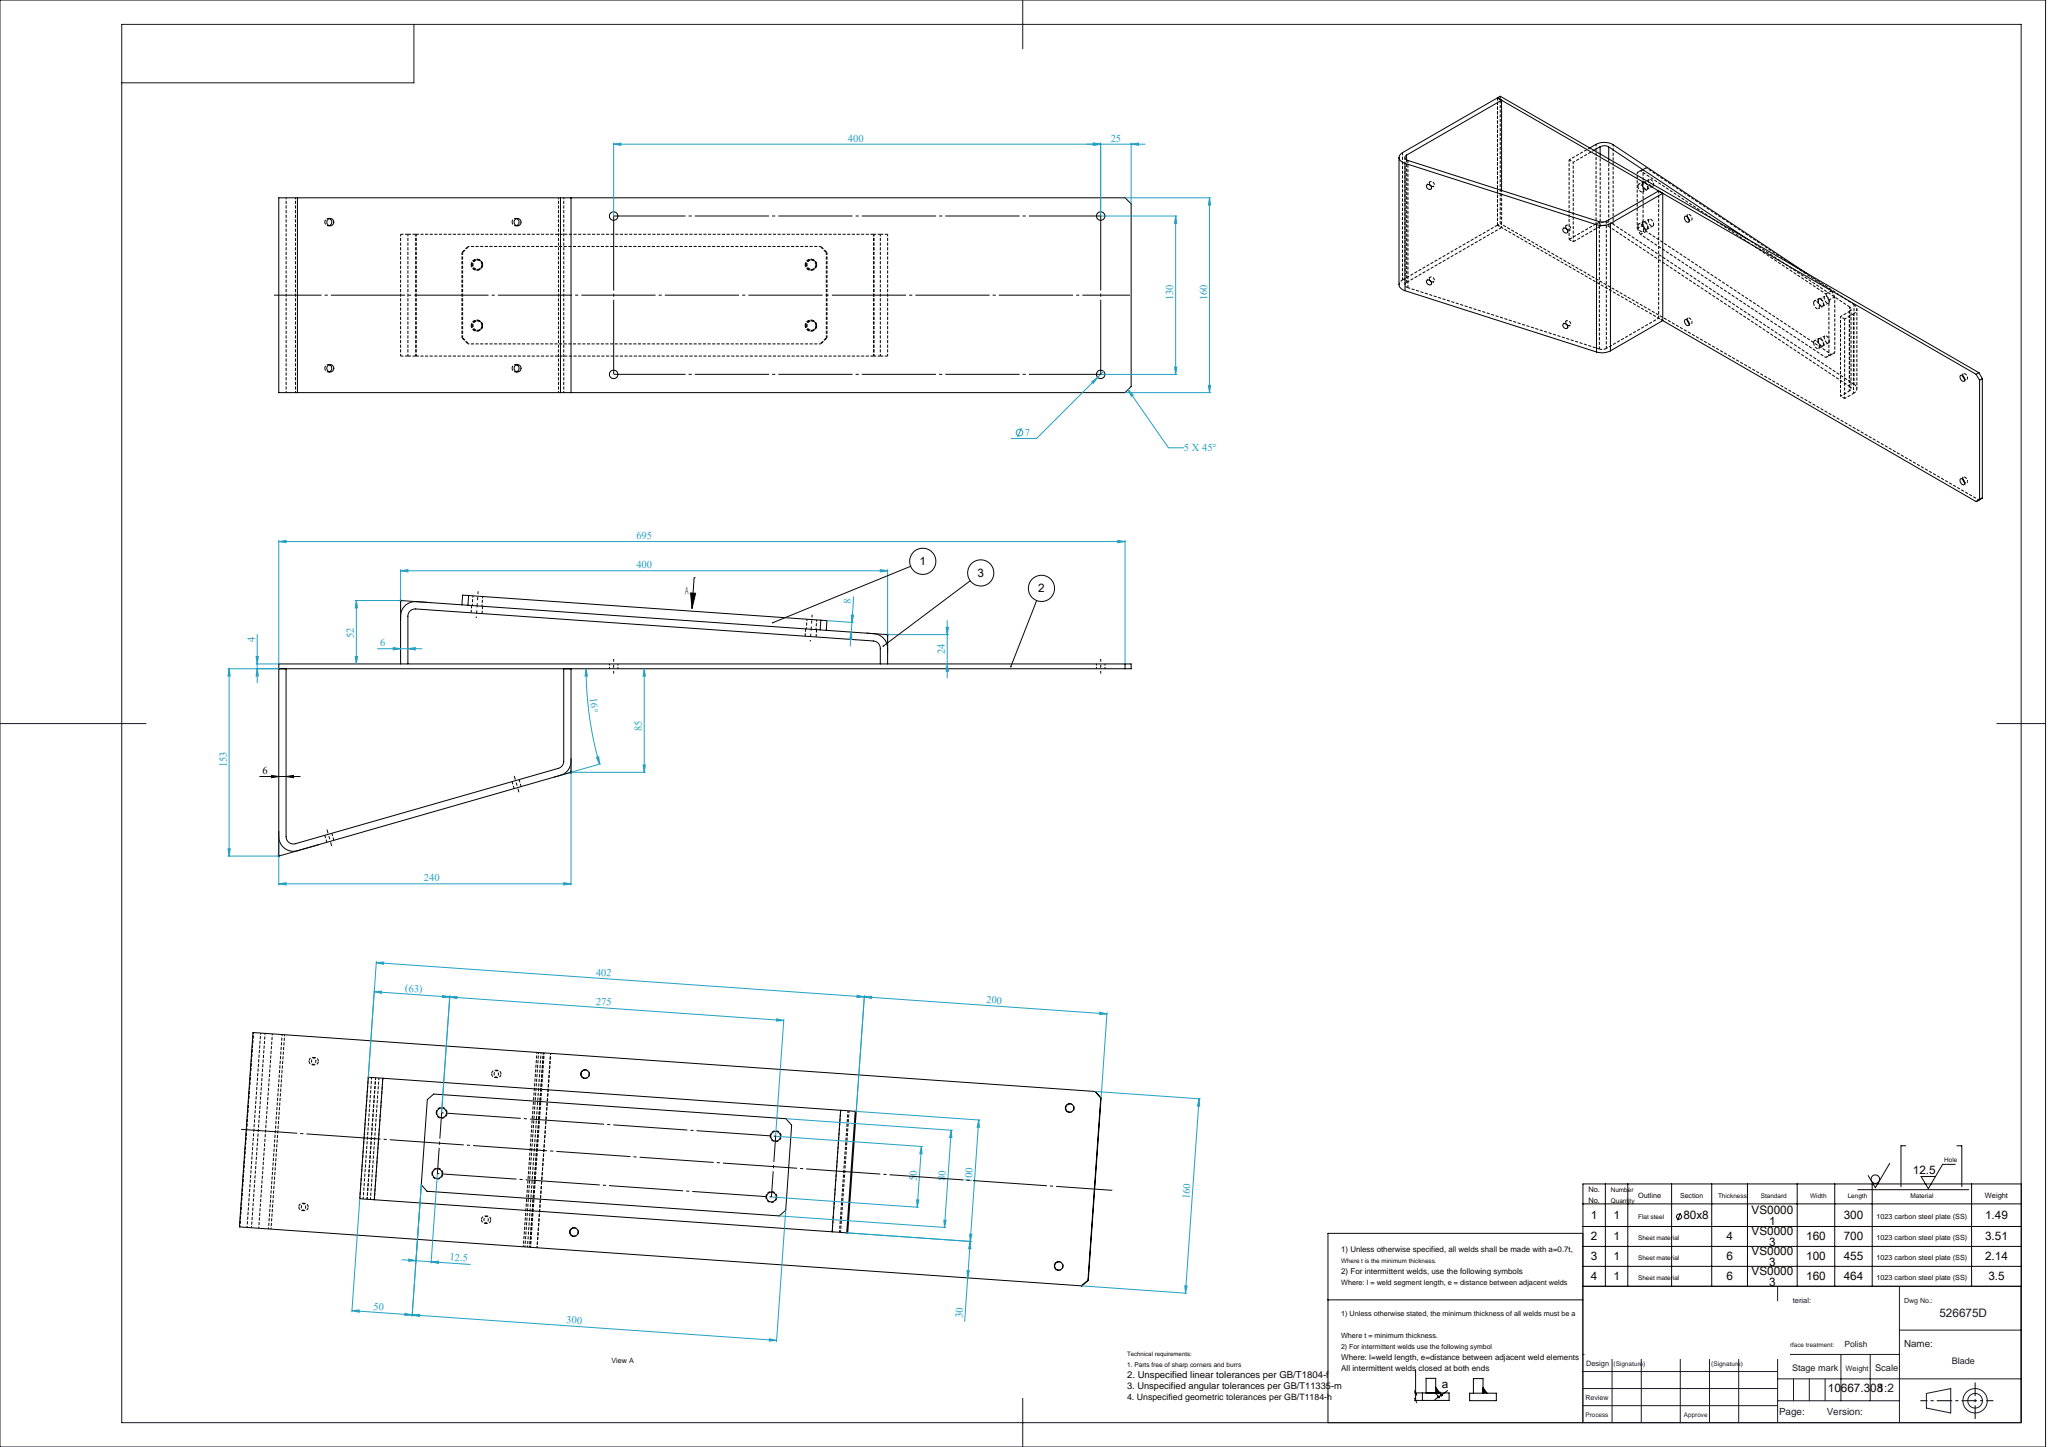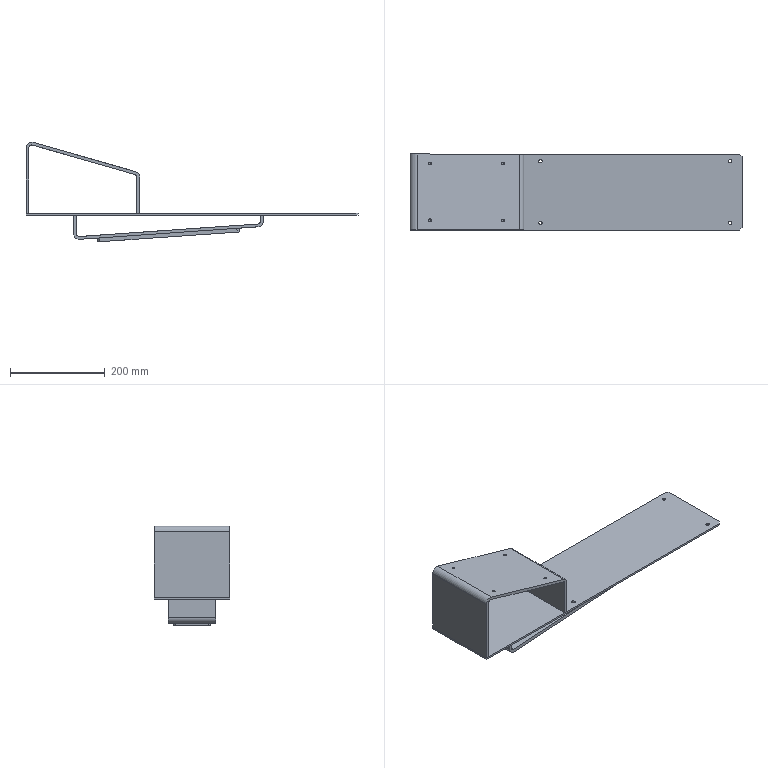Part | SolidWorks | features CompositeCurve 4 | 4 solids | 78 faces | box 700 x 160 x 210.348 mm | volume 1357509 mm3 | cylinder 40 | plane 38 | commonest cylinder face diameters 6 x8 7 x8 8 x8 9 x8 12 x4 24 x4